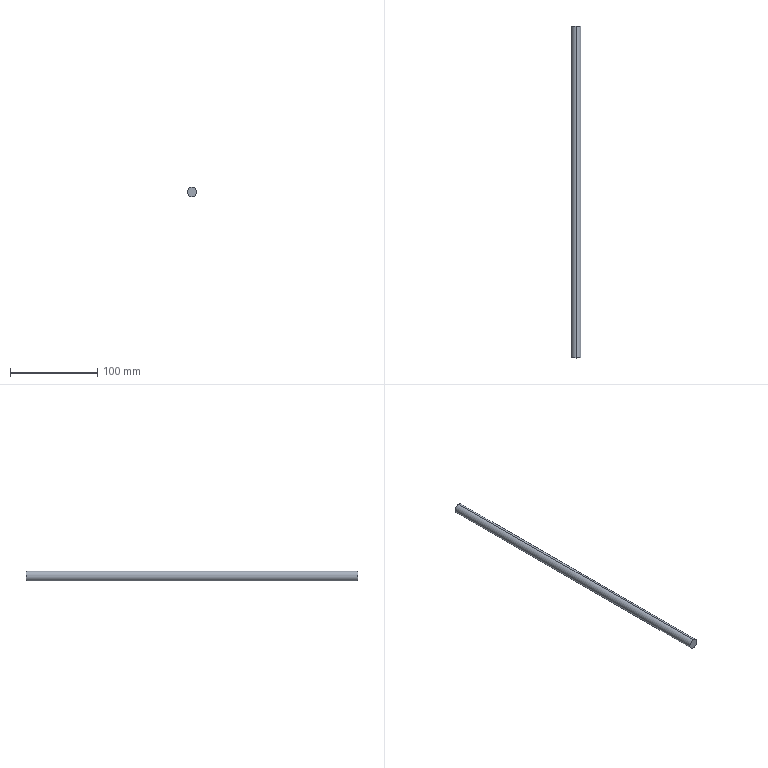Part | STEP file | 4-20.sldasm-Part-353 | 1 solid | 4 faces | box 11.11 x 380 x 11.11 mm | volume 36838 mm3 | cylinder 2 | plane 2 | commonest cylinder face diameters 11.11 x2
STEP:
#1=CARTESIAN_POINT('',(-50.,380.,59.445));
#2=VERTEX_POINT('',#1);
#3=CARTESIAN_POINT('',(-50.,380.,70.555));
#4=VERTEX_POINT('',#3);
#5=CARTESIAN_POINT('',(-50.,380.,65.));
#6=DIRECTION('',(0.,1.,0.));
#7=DIRECTION('',(0.,0.,1.));
#8=AXIS2_PLACEMENT_3D('',#5,#6,#7);
#9=CIRCLE('',#8,5.555);
#10=EDGE_CURVE('',#2,#4,#9,.T.);
#11=ORIENTED_EDGE('',*,*,#10,.F.);
#12=CARTESIAN_POINT('',(-50.,0.,59.445));
#13=VERTEX_POINT('',#12);
#14=CARTESIAN_POINT('',(-50.,430.,59.445));
#15=DIRECTION('',(0.,-1.,0.));
#16=VECTOR('',#15,1000.);
#17=LINE('',#14,#16);
#18=EDGE_CURVE('',#2,#13,#17,.T.);
#19=ORIENTED_EDGE('',*,*,#18,.T.);
#20=CARTESIAN_POINT('',(-50.,0.,70.555));
#21=VERTEX_POINT('',#20);
#22=CARTESIAN_POINT('',(-50.,0.,65.));
#23=DIRECTION('',(0.,1.,0.));
#24=DIRECTION('',(0.,0.,-1.));
#25=AXIS2_PLACEMENT_3D('',#22,#23,#24);
#26=CIRCLE('',#25,5.555);
#27=EDGE_CURVE('',#13,#21,#26,.T.);
#28=ORIENTED_EDGE('',*,*,#27,.T.);
#29=CARTESIAN_POINT('',(-50.,430.,70.555));
#30=DIRECTION('',(0.,-1.,0.));
#31=VECTOR('',#30,1000.);
#32=LINE('',#29,#31);
#33=EDGE_CURVE('',#4,#21,#32,.T.);
#34=ORIENTED_EDGE('',*,*,#33,.F.);
#35=EDGE_LOOP('',(#11,#19,#28,#34));
#36=FACE_OUTER_BOUND('',#35,.T.);
#37=CARTESIAN_POINT('',(-50.,430.,65.));
#38=DIRECTION('',(0.,-1.,0.));
#39=DIRECTION('',(0.,0.,1.));
#40=AXIS2_PLACEMENT_3D('',#37,#38,#39);
#41=CYLINDRICAL_SURFACE('',#40,5.555);
#42=ADVANCED_FACE('',(#36),#41,.T.);
#43=CARTESIAN_POINT('',(-50.,0.,65.));
#44=DIRECTION('',(0.,1.,0.));
#45=DIRECTION('',(0.,0.,-1.));
#46=AXIS2_PLACEMENT_3D('',#43,#44,#45);
#47=CIRCLE('',#46,5.555);
#48=EDGE_CURVE('',#21,#13,#47,.T.);
#49=ORIENTED_EDGE('',*,*,#48,.F.);
#50=ORIENTED_EDGE('',*,*,#27,.F.);
#51=EDGE_LOOP('',(#49,#50));
#52=FACE_OUTER_BOUND('',#51,.T.);
#53=CARTESIAN_POINT('',(-50.,0.,65.));
#54=DIRECTION('',(0.,1.,0.));
#55=DIRECTION('',(0.,0.,-1.));
#56=AXIS2_PLACEMENT_3D('',#53,#54,#55);
#57=PLANE('',#56);
#58=ADVANCED_FACE('',(#52),#57,.F.);
#59=ORIENTED_EDGE('',*,*,#18,.F.);
#60=CARTESIAN_POINT('',(-50.,380.,65.));
#61=DIRECTION('',(0.,1.,0.));
#62=DIRECTION('',(0.,0.,1.));
#63=AXIS2_PLACEMENT_3D('',#60,#61,#62);
#64=CIRCLE('',#63,5.555);
#65=EDGE_CURVE('',#4,#2,#64,.T.);
#66=ORIENTED_EDGE('',*,*,#65,.F.);
#67=ORIENTED_EDGE('',*,*,#33,.T.);
#68=ORIENTED_EDGE('',*,*,#48,.T.);
#69=EDGE_LOOP('',(#59,#66,#67,#68));
#70=FACE_OUTER_BOUND('',#69,.T.);
#71=CARTESIAN_POINT('',(-50.,430.,65.));
#72=DIRECTION('',(0.,-1.,0.));
#73=DIRECTION('',(0.,0.,1.));
#74=AXIS2_PLACEMENT_3D('',#71,#72,#73);
#75=CYLINDRICAL_SURFACE('',#74,5.555);
#76=ADVANCED_FACE('',(#70),#75,.T.);
#77=ORIENTED_EDGE('',*,*,#65,.T.);
#78=ORIENTED_EDGE('',*,*,#10,.T.);
#79=EDGE_LOOP('',(#77,#78));
#80=FACE_OUTER_BOUND('',#79,.T.);
#81=CARTESIAN_POINT('',(125.,380.,90.));
#82=DIRECTION('',(0.,-1.,0.));
#83=DIRECTION('',(0.,0.,1.));
#84=AXIS2_PLACEMENT_3D('',#81,#82,#83);
#85=PLANE('',#84);
#86=ADVANCED_FACE('',(#80),#85,.F.);
#87=CLOSED_SHELL('',(#42,#58,#76,#86));
#88=MANIFOLD_SOLID_BREP('',#87);
#89=CARTESIAN_POINT('',(0.,0.,0.));
#90=DIRECTION('',(0.,0.,1.));
#91=DIRECTION('',(1.,0.,0.));
#92=AXIS2_PLACEMENT_3D('',#89,#90,#91);
#93=(LENGTH_UNIT()NAMED_UNIT(*)SI_UNIT(.MILLI.,.METRE.));
#94=UNCERTAINTY_MEASURE_WITH_UNIT(LENGTH_MEASURE(0.00001),#93,'','');
#95=(NAMED_UNIT(*)PLANE_ANGLE_UNIT()SI_UNIT($,.RADIAN.));
#96=(NAMED_UNIT(*)SI_UNIT($,.STERADIAN.)SOLID_ANGLE_UNIT());
#97=(GEOMETRIC_REPRESENTATION_CONTEXT(3)GLOBAL_UNCERTAINTY_ASSIGNED_CONTEXT((#94))GLOBAL_UNIT_ASSIGNED_CONTEXT((#93,#95,#96))REPRESENTATION_CONTEXT('',''));
#98=ADVANCED_BREP_SHAPE_REPRESENTATION('',(#88,#92),#97);